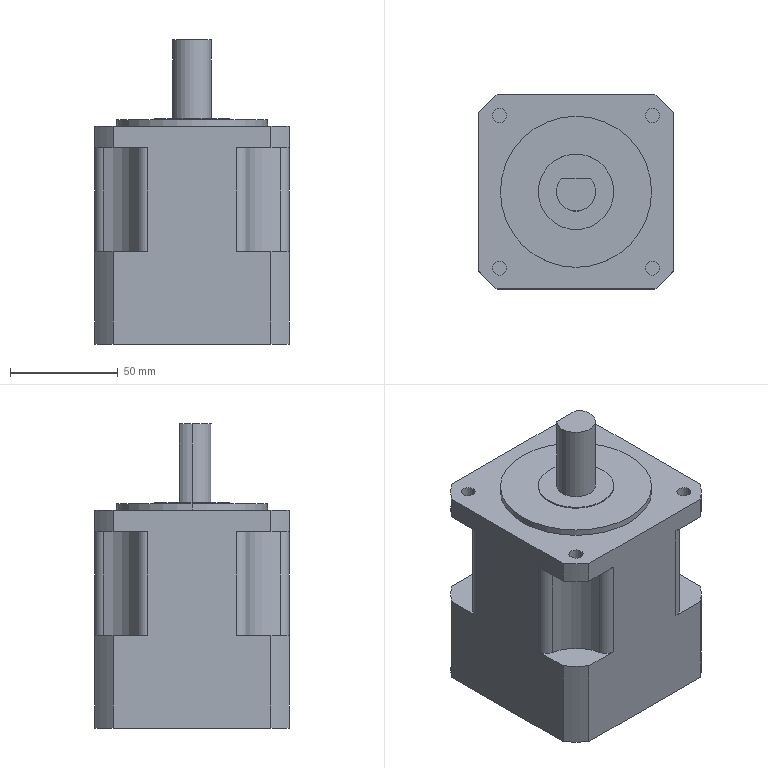Part | SolidWorks | features Boss 4, Cut 3, Extrusion 1, Fillet 1 | 1 solid | 53 faces | box 90 x 90 x 141 mm | volume 768294 mm3 | cylinder 35 | plane 18 | commonest cylinder face diameters 6.5 x8 10 x8 116 x8 40 x4 18 x3 35 x2